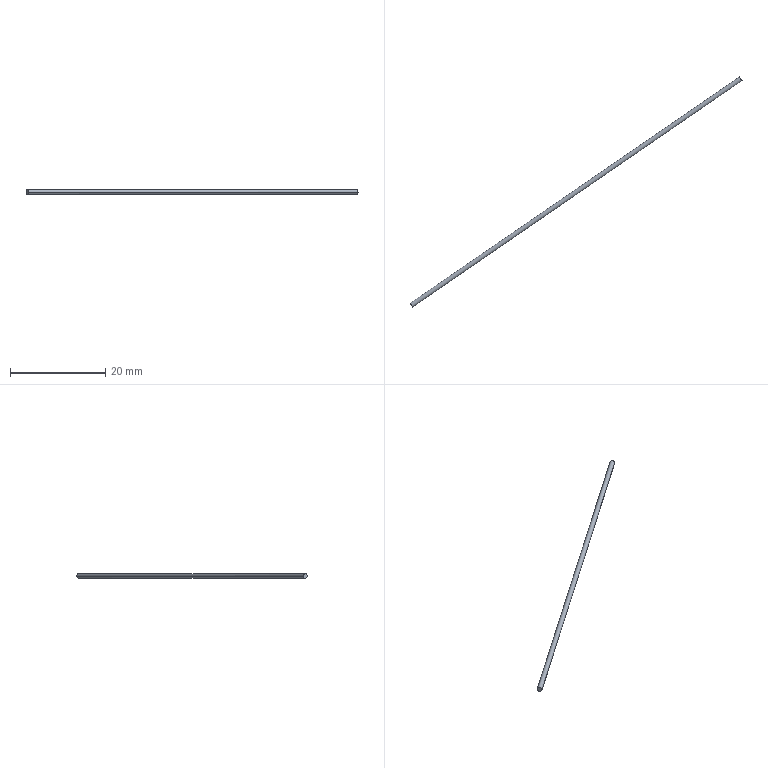Part | STEP file | Termopar-A | 1 solid | 4 faces | box 69.711 x 48.346 x 1 mm | volume 65.873 mm3 | cylinder 2 | plane 2 | commonest cylinder face diameters 1 x2
STEP:
#1=CARTESIAN_POINT('',(0.,0.,0.));
#2=DIRECTION('',(0.,0.,1.));
#3=DIRECTION('',(1.,0.,0.));
#4=AXIS2_PLACEMENT_3D('',#1,#2,#3);
#5=CARTESIAN_POINT('',(-82.696,-56.229,61.55));
#6=VERTEX_POINT('',#5);
#7=CARTESIAN_POINT('',(-82.129,-57.053,61.55));
#8=VERTEX_POINT('',#7);
#9=CARTESIAN_POINT('',(-82.696,-56.229,61.55));
#10=CARTESIAN_POINT('',(-82.696,-56.229,61.681));
#11=CARTESIAN_POINT('',(-82.665,-56.273,61.811));
#12=CARTESIAN_POINT('',(-82.56,-56.426,61.996));
#13=CARTESIAN_POINT('',(-82.487,-56.533,62.05));
#14=CARTESIAN_POINT('',(-82.338,-56.749,62.05));
#15=CARTESIAN_POINT('',(-82.265,-56.856,61.996));
#16=CARTESIAN_POINT('',(-82.16,-57.008,61.811));
#17=CARTESIAN_POINT('',(-82.129,-57.053,61.681));
#18=CARTESIAN_POINT('',(-82.129,-57.053,61.55));
#19=B_SPLINE_CURVE_WITH_KNOTS('',3,(#9,#10,#11,#12,#13,#14,#15,#16,#17,#18),.UNSPECIFIED.,.F.,.F.,(4,2,2,2,4),(0.,0.125,0.25,0.375,0.5),.UNSPECIFIED.);
#20=CARTESIAN_POINT('',(-40.209,-27.635,61.55));
#21=DIRECTION('',(0.8241,0.5664,0.));
#22=DIRECTION('',(-0.5664,0.8241,0.));
#23=AXIS2_PLACEMENT_3D('',#20,#21,#22);
#24=CYLINDRICAL_SURFACE('',#23,0.5);
#25=CARTESIAN_POINT('',(0.,-51.21));
#26=CARTESIAN_POINT('',(0.04757,-51.21));
#27=CARTESIAN_POINT('',(0.1427,-51.21));
#28=CARTESIAN_POINT('',(0.2855,-51.21));
#29=CARTESIAN_POINT('',(0.4284,-51.21));
#30=CARTESIAN_POINT('',(0.5713,-51.21));
#31=CARTESIAN_POINT('',(0.714,-51.21));
#32=CARTESIAN_POINT('',(0.8568,-51.21));
#33=CARTESIAN_POINT('',(0.9995,-51.21));
#34=CARTESIAN_POINT('',(1.142,-51.21));
#35=CARTESIAN_POINT('',(1.285,-51.21));
#36=CARTESIAN_POINT('',(1.428,-51.21));
#37=CARTESIAN_POINT('',(1.571,-51.21));
#38=CARTESIAN_POINT('',(1.714,-51.21));
#39=CARTESIAN_POINT('',(1.856,-51.21));
#40=CARTESIAN_POINT('',(1.999,-51.21));
#41=CARTESIAN_POINT('',(2.142,-51.21));
#42=CARTESIAN_POINT('',(2.285,-51.21));
#43=CARTESIAN_POINT('',(2.428,-51.21));
#44=CARTESIAN_POINT('',(2.57,-51.21));
#45=CARTESIAN_POINT('',(2.713,-51.21));
#46=CARTESIAN_POINT('',(2.856,-51.21));
#47=CARTESIAN_POINT('',(2.999,-51.21));
#48=CARTESIAN_POINT('',(3.094,-51.21));
#49=CARTESIAN_POINT('',(3.142,-51.21));
#50=B_SPLINE_CURVE_WITH_KNOTS('',3,(#25,#26,#27,#28,#29,#30,#31,#32,#33,#34,#35,#36,#37,#38,#39,#40,#41,#42,#43,#44,#45,#46,#47,#48,#49),.UNSPECIFIED.,.F.,.F.,(4,1,1,1,1,1,1,1,1,1,1,1,1,1,1,1,1,1,1,1,1,1,4),(0.,0.02273,0.04545,0.06818,0.09091,0.1136,0.1364,0.1591,0.1818,0.2045,0.2273,0.25,0.2727,0.2955,0.3182,0.3409,0.3636,0.3864,0.4091,0.4318,0.4545,0.4773,0.5),.QUASI_UNIFORM_KNOTS.);
#51=(GEOMETRIC_REPRESENTATION_CONTEXT(2)PARAMETRIC_REPRESENTATION_CONTEXT()REPRESENTATION_CONTEXT('',''));
#52=DEFINITIONAL_REPRESENTATION('',(#50),#51);
#53=PCURVE('',#24,#52);
#54=CARTESIAN_POINT('',(-82.413,-56.641,61.55));
#55=DIRECTION('',(-0.8241,-0.5664,0.));
#56=DIRECTION('',(0.5664,-0.8241,0.));
#57=AXIS2_PLACEMENT_3D('',#54,#55,#56);
#58=PLANE('',#57);
#59=CARTESIAN_POINT('',(-0.5,0.));
#60=CARTESIAN_POINT('',(-0.5,0.1309));
#61=CARTESIAN_POINT('',(-0.4461,0.261));
#62=CARTESIAN_POINT('',(-0.261,0.4461));
#63=CARTESIAN_POINT('',(-0.1309,0.5));
#64=CARTESIAN_POINT('',(0.1309,0.5));
#65=CARTESIAN_POINT('',(0.261,0.4461));
#66=CARTESIAN_POINT('',(0.4461,0.261));
#67=CARTESIAN_POINT('',(0.5,0.1309));
#68=CARTESIAN_POINT('',(0.5,0.));
#69=B_SPLINE_CURVE_WITH_KNOTS('',3,(#59,#60,#61,#62,#63,#64,#65,#66,#67,#68),.UNSPECIFIED.,.F.,.F.,(4,2,2,2,4),(0.,0.125,0.25,0.375,0.5),.UNSPECIFIED.);
#70=(GEOMETRIC_REPRESENTATION_CONTEXT(2)PARAMETRIC_REPRESENTATION_CONTEXT()REPRESENTATION_CONTEXT('',''));
#71=DEFINITIONAL_REPRESENTATION('',(#69),#70);
#72=PCURVE('',#58,#71);
#73=SURFACE_CURVE('',#19,(#53,#72),.PCURVE_S1.);
#74=EDGE_CURVE('',#6,#8,#73,.T.);
#75=ORIENTED_EDGE('',*,*,#74,.T.);
#76=CARTESIAN_POINT('',(-12.985,-9.531,61.55));
#77=VERTEX_POINT('',#76);
#78=CARTESIAN_POINT('',(-39.926,-28.047,61.55));
#79=DIRECTION('',(0.8241,0.5664,0.));
#80=VECTOR('',#79,1.);
#81=LINE('',#78,#80);
#82=CARTESIAN_POINT('',(3.142,0.));
#83=DIRECTION('',(0.,1.));
#84=VECTOR('',#83,1.);
#85=LINE('',#82,#84);
#86=(GEOMETRIC_REPRESENTATION_CONTEXT(2)PARAMETRIC_REPRESENTATION_CONTEXT()REPRESENTATION_CONTEXT('',''));
#87=DEFINITIONAL_REPRESENTATION('',(#85),#86);
#88=PCURVE('',#24,#87);
#89=CARTESIAN_POINT('',(-40.209,-27.635,61.55));
#90=DIRECTION('',(0.8241,0.5664,0.));
#91=DIRECTION('',(-0.5664,0.8241,0.));
#92=AXIS2_PLACEMENT_3D('',#89,#90,#91);
#93=CYLINDRICAL_SURFACE('',#92,0.5);
#94=CARTESIAN_POINT('',(3.142,0.));
#95=DIRECTION('',(0.,1.));
#96=VECTOR('',#95,1.);
#97=LINE('',#94,#96);
#98=(GEOMETRIC_REPRESENTATION_CONTEXT(2)PARAMETRIC_REPRESENTATION_CONTEXT()REPRESENTATION_CONTEXT('',''));
#99=DEFINITIONAL_REPRESENTATION('',(#97),#98);
#100=PCURVE('',#93,#99);
#101=SURFACE_CURVE('',#81,(#88,#100),.PCURVE_S1.);
#102=EDGE_CURVE('',#8,#77,#101,.T.);
#103=ORIENTED_EDGE('',*,*,#102,.T.);
#104=CARTESIAN_POINT('',(-13.552,-8.707,61.55));
#105=VERTEX_POINT('',#104);
#106=CARTESIAN_POINT('',(-12.985,-9.531,61.55));
#107=CARTESIAN_POINT('',(-12.985,-9.531,61.681));
#108=CARTESIAN_POINT('',(-13.016,-9.487,61.811));
#109=CARTESIAN_POINT('',(-13.121,-9.334,61.996));
#110=CARTESIAN_POINT('',(-13.194,-9.227,62.05));
#111=CARTESIAN_POINT('',(-13.343,-9.011,62.05));
#112=CARTESIAN_POINT('',(-13.416,-8.904,61.996));
#113=CARTESIAN_POINT('',(-13.521,-8.751,61.811));
#114=CARTESIAN_POINT('',(-13.552,-8.707,61.681));
#115=CARTESIAN_POINT('',(-13.552,-8.707,61.55));
#116=B_SPLINE_CURVE_WITH_KNOTS('',3,(#106,#107,#108,#109,#110,#111,#112,#113,#114,#115),.UNSPECIFIED.,.F.,.F.,(4,2,2,2,4),(0.5,0.625,0.75,0.875,1.),.UNSPECIFIED.);
#117=CARTESIAN_POINT('',(3.142,32.69));
#118=CARTESIAN_POINT('',(3.094,32.69));
#119=CARTESIAN_POINT('',(2.999,32.69));
#120=CARTESIAN_POINT('',(2.856,32.69));
#121=CARTESIAN_POINT('',(2.713,32.69));
#122=CARTESIAN_POINT('',(2.57,32.69));
#123=CARTESIAN_POINT('',(2.428,32.69));
#124=CARTESIAN_POINT('',(2.285,32.69));
#125=CARTESIAN_POINT('',(2.142,32.69));
#126=CARTESIAN_POINT('',(1.999,32.69));
#127=CARTESIAN_POINT('',(1.856,32.69));
#128=CARTESIAN_POINT('',(1.714,32.69));
#129=CARTESIAN_POINT('',(1.571,32.69));
#130=CARTESIAN_POINT('',(1.428,32.69));
#131=CARTESIAN_POINT('',(1.285,32.69));
#132=CARTESIAN_POINT('',(1.142,32.69));
#133=CARTESIAN_POINT('',(0.9995,32.69));
#134=CARTESIAN_POINT('',(0.8568,32.69));
#135=CARTESIAN_POINT('',(0.714,32.69));
#136=CARTESIAN_POINT('',(0.5713,32.69));
#137=CARTESIAN_POINT('',(0.4284,32.69));
#138=CARTESIAN_POINT('',(0.2855,32.69));
#139=CARTESIAN_POINT('',(0.1427,32.69));
#140=CARTESIAN_POINT('',(0.04757,32.69));
#141=CARTESIAN_POINT('',(0.,32.69));
#142=B_SPLINE_CURVE_WITH_KNOTS('',3,(#117,#118,#119,#120,#121,#122,#123,#124,#125,#126,#127,#128,#129,#130,#131,#132,#133,#134,#135,#136,#137,#138,#139,#140,#141),.UNSPECIFIED.,.F.,.F.,(4,1,1,1,1,1,1,1,1,1,1,1,1,1,1,1,1,1,1,1,1,1,4),(0.5,0.5227,0.5455,0.5682,0.5909,0.6136,0.6364,0.6591,0.6818,0.7045,0.7273,0.75,0.7727,0.7955,0.8182,0.8409,0.8636,0.8864,0.9091,0.9318,0.9545,0.9773,1.),.QUASI_UNIFORM_KNOTS.);
#143=(GEOMETRIC_REPRESENTATION_CONTEXT(2)PARAMETRIC_REPRESENTATION_CONTEXT()REPRESENTATION_CONTEXT('',''));
#144=DEFINITIONAL_REPRESENTATION('',(#142),#143);
#145=PCURVE('',#24,#144);
#146=CARTESIAN_POINT('',(-13.268,-9.119,61.55));
#147=DIRECTION('',(-0.8241,-0.5664,0.));
#148=DIRECTION('',(0.5664,-0.8241,0.));
#149=AXIS2_PLACEMENT_3D('',#146,#147,#148);
#150=PLANE('',#149);
#151=CARTESIAN_POINT('',(0.5,0.));
#152=CARTESIAN_POINT('',(0.5,0.1309));
#153=CARTESIAN_POINT('',(0.4461,0.261));
#154=CARTESIAN_POINT('',(0.261,0.4461));
#155=CARTESIAN_POINT('',(0.1309,0.5));
#156=CARTESIAN_POINT('',(-0.1309,0.5));
#157=CARTESIAN_POINT('',(-0.261,0.4461));
#158=CARTESIAN_POINT('',(-0.4461,0.261));
#159=CARTESIAN_POINT('',(-0.5,0.1309));
#160=CARTESIAN_POINT('',(-0.5,0.));
#161=B_SPLINE_CURVE_WITH_KNOTS('',3,(#151,#152,#153,#154,#155,#156,#157,#158,#159,#160),.UNSPECIFIED.,.F.,.F.,(4,2,2,2,4),(0.5,0.625,0.75,0.875,1.),.UNSPECIFIED.);
#162=(GEOMETRIC_REPRESENTATION_CONTEXT(2)PARAMETRIC_REPRESENTATION_CONTEXT()REPRESENTATION_CONTEXT('',''));
#163=DEFINITIONAL_REPRESENTATION('',(#161),#162);
#164=PCURVE('',#150,#163);
#165=SURFACE_CURVE('',#116,(#145,#164),.PCURVE_S1.);
#166=EDGE_CURVE('',#77,#105,#165,.T.);
#167=ORIENTED_EDGE('',*,*,#166,.T.);
#168=CARTESIAN_POINT('',(-40.492,-27.223,61.55));
#169=DIRECTION('',(0.8241,0.5664,0.));
#170=VECTOR('',#169,1.);
#171=LINE('',#168,#170);
#172=CARTESIAN_POINT('',(0.,0.));
#173=DIRECTION('',(0.,1.));
#174=VECTOR('',#173,1.);
#175=LINE('',#172,#174);
#176=(GEOMETRIC_REPRESENTATION_CONTEXT(2)PARAMETRIC_REPRESENTATION_CONTEXT()REPRESENTATION_CONTEXT('',''));
#177=DEFINITIONAL_REPRESENTATION('',(#175),#176);
#178=PCURVE('',#24,#177);
#179=CARTESIAN_POINT('',(6.283,0.));
#180=DIRECTION('',(0.,1.));
#181=VECTOR('',#180,1.);
#182=LINE('',#179,#181);
#183=(GEOMETRIC_REPRESENTATION_CONTEXT(2)PARAMETRIC_REPRESENTATION_CONTEXT()REPRESENTATION_CONTEXT('',''));
#184=DEFINITIONAL_REPRESENTATION('',(#182),#183);
#185=PCURVE('',#93,#184);
#186=SURFACE_CURVE('',#171,(#178,#185),.PCURVE_S1.);
#187=EDGE_CURVE('',#6,#105,#186,.T.);
#188=ORIENTED_EDGE('',*,*,#187,.F.);
#189=EDGE_LOOP('',(#75,#103,#167,#188));
#190=FACE_BOUND('',#189,.T.);
#191=ADVANCED_FACE('',(#190),#24,.T.);
#192=ORIENTED_EDGE('',*,*,#102,.F.);
#193=CARTESIAN_POINT('',(-82.129,-57.053,61.55));
#194=CARTESIAN_POINT('',(-82.129,-57.053,61.419));
#195=CARTESIAN_POINT('',(-82.16,-57.008,61.289));
#196=CARTESIAN_POINT('',(-82.265,-56.856,61.104));
#197=CARTESIAN_POINT('',(-82.338,-56.749,61.05));
#198=CARTESIAN_POINT('',(-82.487,-56.533,61.05));
#199=CARTESIAN_POINT('',(-82.56,-56.426,61.104));
#200=CARTESIAN_POINT('',(-82.665,-56.273,61.289));
#201=CARTESIAN_POINT('',(-82.696,-56.229,61.419));
#202=CARTESIAN_POINT('',(-82.696,-56.229,61.55));
#203=B_SPLINE_CURVE_WITH_KNOTS('',3,(#193,#194,#195,#196,#197,#198,#199,#200,#201,#202),.UNSPECIFIED.,.F.,.F.,(4,2,2,2,4),(0.5,0.625,0.75,0.875,1.),.UNSPECIFIED.);
#204=CARTESIAN_POINT('',(3.142,-51.21));
#205=CARTESIAN_POINT('',(3.189,-51.21));
#206=CARTESIAN_POINT('',(3.284,-51.21));
#207=CARTESIAN_POINT('',(3.427,-51.21));
#208=CARTESIAN_POINT('',(3.57,-51.21));
#209=CARTESIAN_POINT('',(3.713,-51.21));
#210=CARTESIAN_POINT('',(3.856,-51.21));
#211=CARTESIAN_POINT('',(3.998,-51.21));
#212=CARTESIAN_POINT('',(4.141,-51.21));
#213=CARTESIAN_POINT('',(4.284,-51.21));
#214=CARTESIAN_POINT('',(4.427,-51.21));
#215=CARTESIAN_POINT('',(4.57,-51.21));
#216=CARTESIAN_POINT('',(4.712,-51.21));
#217=CARTESIAN_POINT('',(4.855,-51.21));
#218=CARTESIAN_POINT('',(4.998,-51.21));
#219=CARTESIAN_POINT('',(5.141,-51.21));
#220=CARTESIAN_POINT('',(5.284,-51.21));
#221=CARTESIAN_POINT('',(5.426,-51.21));
#222=CARTESIAN_POINT('',(5.569,-51.21));
#223=CARTESIAN_POINT('',(5.712,-51.21));
#224=CARTESIAN_POINT('',(5.855,-51.21));
#225=CARTESIAN_POINT('',(5.998,-51.21));
#226=CARTESIAN_POINT('',(6.14,-51.21));
#227=CARTESIAN_POINT('',(6.236,-51.21));
#228=CARTESIAN_POINT('',(6.283,-51.21));
#229=B_SPLINE_CURVE_WITH_KNOTS('',3,(#204,#205,#206,#207,#208,#209,#210,#211,#212,#213,#214,#215,#216,#217,#218,#219,#220,#221,#222,#223,#224,#225,#226,#227,#228),.UNSPECIFIED.,.F.,.F.,(4,1,1,1,1,1,1,1,1,1,1,1,1,1,1,1,1,1,1,1,1,1,4),(0.5,0.5227,0.5455,0.5682,0.5909,0.6136,0.6364,0.6591,0.6818,0.7045,0.7273,0.75,0.7727,0.7955,0.8182,0.8409,0.8636,0.8864,0.9091,0.9318,0.9545,0.9773,1.),.QUASI_UNIFORM_KNOTS.);
#230=(GEOMETRIC_REPRESENTATION_CONTEXT(2)PARAMETRIC_REPRESENTATION_CONTEXT()REPRESENTATION_CONTEXT('',''));
#231=DEFINITIONAL_REPRESENTATION('',(#229),#230);
#232=PCURVE('',#93,#231);
#233=CARTESIAN_POINT('',(0.5,0.));
#234=CARTESIAN_POINT('',(0.5,-0.1309));
#235=CARTESIAN_POINT('',(0.4461,-0.261));
#236=CARTESIAN_POINT('',(0.261,-0.4461));
#237=CARTESIAN_POINT('',(0.1309,-0.5));
#238=CARTESIAN_POINT('',(-0.1309,-0.5));
#239=CARTESIAN_POINT('',(-0.261,-0.4461));
#240=CARTESIAN_POINT('',(-0.4461,-0.261));
#241=CARTESIAN_POINT('',(-0.5,-0.1309));
#242=CARTESIAN_POINT('',(-0.5,0.));
#243=B_SPLINE_CURVE_WITH_KNOTS('',3,(#233,#234,#235,#236,#237,#238,#239,#240,#241,#242),.UNSPECIFIED.,.F.,.F.,(4,2,2,2,4),(0.5,0.625,0.75,0.875,1.),.UNSPECIFIED.);
#244=(GEOMETRIC_REPRESENTATION_CONTEXT(2)PARAMETRIC_REPRESENTATION_CONTEXT()REPRESENTATION_CONTEXT('',''));
#245=DEFINITIONAL_REPRESENTATION('',(#243),#244);
#246=PCURVE('',#58,#245);
#247=SURFACE_CURVE('',#203,(#232,#246),.PCURVE_S1.);
#248=EDGE_CURVE('',#8,#6,#247,.T.);
#249=ORIENTED_EDGE('',*,*,#248,.T.);
#250=ORIENTED_EDGE('',*,*,#187,.T.);
#251=CARTESIAN_POINT('',(-13.552,-8.707,61.55));
#252=CARTESIAN_POINT('',(-13.552,-8.707,61.419));
#253=CARTESIAN_POINT('',(-13.521,-8.751,61.289));
#254=CARTESIAN_POINT('',(-13.416,-8.904,61.104));
#255=CARTESIAN_POINT('',(-13.343,-9.011,61.05));
#256=CARTESIAN_POINT('',(-13.194,-9.227,61.05));
#257=CARTESIAN_POINT('',(-13.121,-9.334,61.104));
#258=CARTESIAN_POINT('',(-13.016,-9.487,61.289));
#259=CARTESIAN_POINT('',(-12.985,-9.531,61.419));
#260=CARTESIAN_POINT('',(-12.985,-9.531,61.55));
#261=B_SPLINE_CURVE_WITH_KNOTS('',3,(#251,#252,#253,#254,#255,#256,#257,#258,#259,#260),.UNSPECIFIED.,.F.,.F.,(4,2,2,2,4),(0.,0.125,0.25,0.375,0.5),.UNSPECIFIED.);
#262=CARTESIAN_POINT('',(6.283,32.69));
#263=CARTESIAN_POINT('',(6.236,32.69));
#264=CARTESIAN_POINT('',(6.14,32.69));
#265=CARTESIAN_POINT('',(5.998,32.69));
#266=CARTESIAN_POINT('',(5.855,32.69));
#267=CARTESIAN_POINT('',(5.712,32.69));
#268=CARTESIAN_POINT('',(5.569,32.69));
#269=CARTESIAN_POINT('',(5.426,32.69));
#270=CARTESIAN_POINT('',(5.284,32.69));
#271=CARTESIAN_POINT('',(5.141,32.69));
#272=CARTESIAN_POINT('',(4.998,32.69));
#273=CARTESIAN_POINT('',(4.855,32.69));
#274=CARTESIAN_POINT('',(4.712,32.69));
#275=CARTESIAN_POINT('',(4.57,32.69));
#276=CARTESIAN_POINT('',(4.427,32.69));
#277=CARTESIAN_POINT('',(4.284,32.69));
#278=CARTESIAN_POINT('',(4.141,32.69));
#279=CARTESIAN_POINT('',(3.998,32.69));
#280=CARTESIAN_POINT('',(3.856,32.69));
#281=CARTESIAN_POINT('',(3.713,32.69));
#282=CARTESIAN_POINT('',(3.57,32.69));
#283=CARTESIAN_POINT('',(3.427,32.69));
#284=CARTESIAN_POINT('',(3.284,32.69));
#285=CARTESIAN_POINT('',(3.189,32.69));
#286=CARTESIAN_POINT('',(3.142,32.69));
#287=B_SPLINE_CURVE_WITH_KNOTS('',3,(#262,#263,#264,#265,#266,#267,#268,#269,#270,#271,#272,#273,#274,#275,#276,#277,#278,#279,#280,#281,#282,#283,#284,#285,#286),.UNSPECIFIED.,.F.,.F.,(4,1,1,1,1,1,1,1,1,1,1,1,1,1,1,1,1,1,1,1,1,1,4),(0.,0.02273,0.04545,0.06818,0.09091,0.1136,0.1364,0.1591,0.1818,0.2045,0.2273,0.25,0.2727,0.2955,0.3182,0.3409,0.3636,0.3864,0.4091,0.4318,0.4545,0.4773,0.5),.QUASI_UNIFORM_KNOTS.);
#288=(GEOMETRIC_REPRESENTATION_CONTEXT(2)PARAMETRIC_REPRESENTATION_CONTEXT()REPRESENTATION_CONTEXT('',''));
#289=DEFINITIONAL_REPRESENTATION('',(#287),#288);
#290=PCURVE('',#93,#289);
#291=CARTESIAN_POINT('',(-0.5,0.));
#292=CARTESIAN_POINT('',(-0.5,-0.1309));
#293=CARTESIAN_POINT('',(-0.4461,-0.261));
#294=CARTESIAN_POINT('',(-0.261,-0.4461));
#295=CARTESIAN_POINT('',(-0.1309,-0.5));
#296=CARTESIAN_POINT('',(0.1309,-0.5));
#297=CARTESIAN_POINT('',(0.261,-0.4461));
#298=CARTESIAN_POINT('',(0.4461,-0.261));
#299=CARTESIAN_POINT('',(0.5,-0.1309));
#300=CARTESIAN_POINT('',(0.5,0.));
#301=B_SPLINE_CURVE_WITH_KNOTS('',3,(#291,#292,#293,#294,#295,#296,#297,#298,#299,#300),.UNSPECIFIED.,.F.,.F.,(4,2,2,2,4),(0.,0.125,0.25,0.375,0.5),.UNSPECIFIED.);
#302=(GEOMETRIC_REPRESENTATION_CONTEXT(2)PARAMETRIC_REPRESENTATION_CONTEXT()REPRESENTATION_CONTEXT('',''));
#303=DEFINITIONAL_REPRESENTATION('',(#301),#302);
#304=PCURVE('',#150,#303);
#305=SURFACE_CURVE('',#261,(#290,#304),.PCURVE_S1.);
#306=EDGE_CURVE('',#105,#77,#305,.T.);
#307=ORIENTED_EDGE('',*,*,#306,.T.);
#308=EDGE_LOOP('',(#192,#249,#250,#307));
#309=FACE_BOUND('',#308,.T.);
#310=ADVANCED_FACE('',(#309),#93,.T.);
#311=ORIENTED_EDGE('',*,*,#74,.F.);
#312=ORIENTED_EDGE('',*,*,#248,.F.);
#313=EDGE_LOOP('',(#311,#312));
#314=FACE_BOUND('',#313,.T.);
#315=ADVANCED_FACE('',(#314),#58,.T.);
#316=ORIENTED_EDGE('',*,*,#306,.F.);
#317=ORIENTED_EDGE('',*,*,#166,.F.);
#318=EDGE_LOOP('',(#316,#317));
#319=FACE_BOUND('',#318,.T.);
#320=ADVANCED_FACE('',(#319),#150,.F.);
#321=CLOSED_SHELL('',(#191,#310,#315,#320));
#322=MANIFOLD_SOLID_BREP('',#321);
#323=(LENGTH_UNIT()NAMED_UNIT(*)SI_UNIT(.MILLI.,.METRE.));
#324=UNCERTAINTY_MEASURE_WITH_UNIT(LENGTH_MEASURE(0.0005),#323,'','');
#325=(NAMED_UNIT(*)PLANE_ANGLE_UNIT()SI_UNIT($,.RADIAN.));
#326=(NAMED_UNIT(*)SI_UNIT($,.STERADIAN.)SOLID_ANGLE_UNIT());
#327=(GEOMETRIC_REPRESENTATION_CONTEXT(3)GLOBAL_UNCERTAINTY_ASSIGNED_CONTEXT((#324))GLOBAL_UNIT_ASSIGNED_CONTEXT((#323,#325,#326))REPRESENTATION_CONTEXT('',''));
#328=ADVANCED_BREP_SHAPE_REPRESENTATION('',(#4,#322),#327);